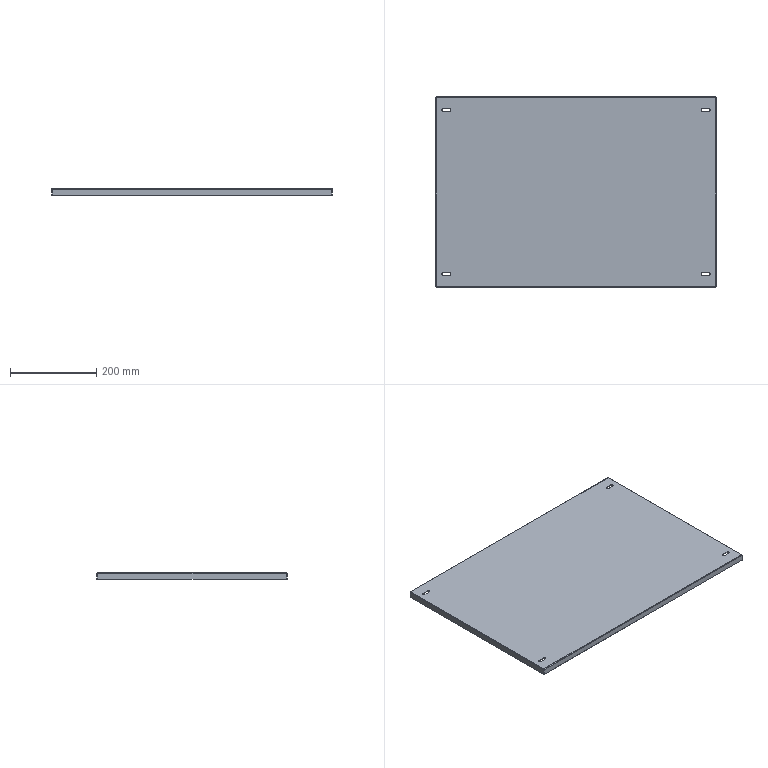Part | STEP file | FHD-021-002 electrical mounting plate | 1 solid | 54 faces | box 650 x 440 x 15 mm | volume 470822 mm3 | plane 30 | cylinder 16 | spline 8 | commonest cylinder face diameters 6 x8 0.4 x4 3.4 x4